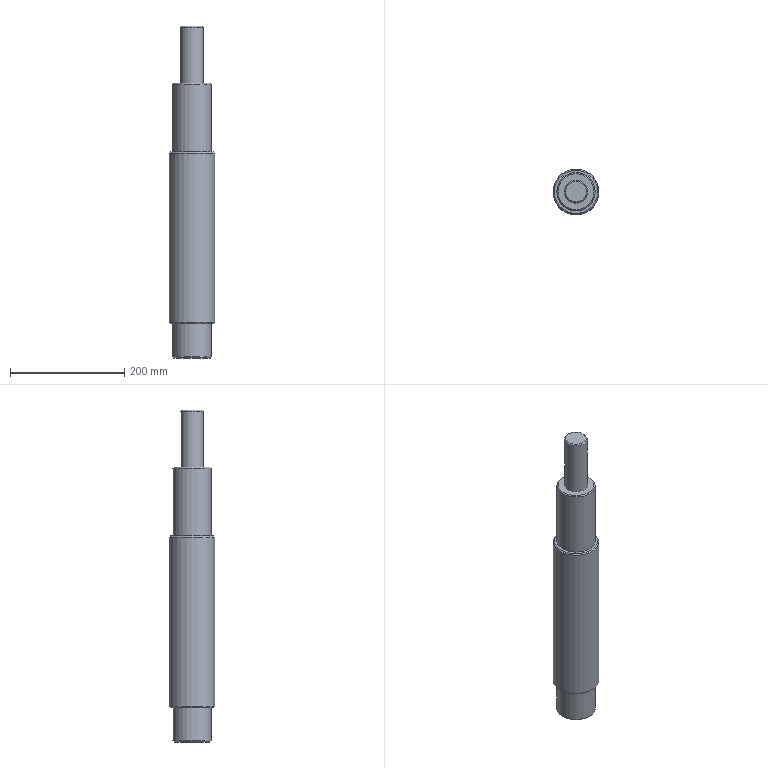Part | NX | features CYLINDER 4, CHAMFER 1, DATUM_CSYS 1 | 1 solid | 14 faces | box 80 x 80 x 580 mm | volume 2266189 mm3 | plane 5 | cone 5 | cylinder 4 | commonest cylinder face diameters 67 x2 40 x1 80 x1
STEP:
#1=CARTESIAN_POINT('',(-31.5,0.,0.));
#2=VERTEX_POINT('',#1);
#3=CARTESIAN_POINT('',(0.,0.,0.));
#4=DIRECTION('',(0.,0.,-1.));
#5=DIRECTION('',(-1.,0.,0.));
#6=AXIS2_PLACEMENT_3D('',#3,#4,#5);
#7=CIRCLE('',#6,31.5);
#8=EDGE_CURVE('',#2,#2,#7,.T.);
#9=ORIENTED_EDGE('',*,*,#8,.T.);
#10=EDGE_LOOP('',(#9));
#11=FACE_BOUND('',#10,.T.);
#12=CARTESIAN_POINT('',(0.,0.,0.));
#13=DIRECTION('',(0.,0.,-1.));
#14=DIRECTION('',(-1.,0.,0.));
#15=AXIS2_PLACEMENT_3D('',#12,#13,#14);
#16=PLANE('',#15);
#17=ADVANCED_FACE('',(#11),#16,.T.);
#18=CARTESIAN_POINT('',(-33.5,0.,2.));
#19=VERTEX_POINT('',#18);
#20=CARTESIAN_POINT('',(0.,0.,2.));
#21=DIRECTION('',(0.,0.,-1.));
#22=DIRECTION('',(-1.,0.,0.));
#23=AXIS2_PLACEMENT_3D('',#20,#21,#22);
#24=CIRCLE('',#23,33.5);
#25=EDGE_CURVE('',#19,#19,#24,.F.);
#26=ORIENTED_EDGE('',*,*,#25,.T.);
#27=EDGE_LOOP('',(#26));
#28=FACE_BOUND('',#27,.T.);
#29=CARTESIAN_POINT('',(-33.5,0.,60.));
#30=VERTEX_POINT('',#29);
#31=CARTESIAN_POINT('',(0.,0.,60.));
#32=DIRECTION('',(0.,0.,-1.));
#33=DIRECTION('',(-1.,0.,0.));
#34=AXIS2_PLACEMENT_3D('',#31,#32,#33);
#35=CIRCLE('',#34,33.5);
#36=EDGE_CURVE('',#30,#30,#35,.F.);
#37=ORIENTED_EDGE('',*,*,#36,.F.);
#38=EDGE_LOOP('',(#37));
#39=FACE_BOUND('',#38,.T.);
#40=CARTESIAN_POINT('',(0.,0.,0.));
#41=DIRECTION('',(0.,0.,1.));
#42=DIRECTION('',(1.,0.,0.));
#43=AXIS2_PLACEMENT_3D('',#40,#41,#42);
#44=CYLINDRICAL_SURFACE('',#43,33.5);
#45=ADVANCED_FACE('',(#28,#39),#44,.T.);
#46=CARTESIAN_POINT('',(38.,0.,360.));
#47=VERTEX_POINT('',#46);
#48=CARTESIAN_POINT('',(0.,0.,360.));
#49=DIRECTION('',(0.,0.,1.));
#50=DIRECTION('',(1.,0.,0.));
#51=AXIS2_PLACEMENT_3D('',#48,#49,#50);
#52=CIRCLE('',#51,38.);
#53=EDGE_CURVE('',#47,#47,#52,.T.);
#54=ORIENTED_EDGE('',*,*,#53,.T.);
#55=EDGE_LOOP('',(#54));
#56=FACE_BOUND('',#55,.T.);
#57=CARTESIAN_POINT('',(33.5,0.,360.));
#58=VERTEX_POINT('',#57);
#59=CARTESIAN_POINT('',(0.,0.,360.));
#60=DIRECTION('',(0.,0.,1.));
#61=DIRECTION('',(1.,0.,0.));
#62=AXIS2_PLACEMENT_3D('',#59,#60,#61);
#63=CIRCLE('',#62,33.5);
#64=EDGE_CURVE('',#58,#58,#63,.T.);
#65=ORIENTED_EDGE('',*,*,#64,.F.);
#66=EDGE_LOOP('',(#65));
#67=FACE_BOUND('',#66,.T.);
#68=CARTESIAN_POINT('',(0.,0.,360.));
#69=DIRECTION('',(0.,0.,1.));
#70=DIRECTION('',(1.,0.,0.));
#71=AXIS2_PLACEMENT_3D('',#68,#69,#70);
#72=PLANE('',#71);
#73=ADVANCED_FACE('',(#56,#67),#72,.T.);
#74=CARTESIAN_POINT('',(-38.,0.,60.));
#75=VERTEX_POINT('',#74);
#76=CARTESIAN_POINT('',(0.,0.,60.));
#77=DIRECTION('',(0.,0.,-1.));
#78=DIRECTION('',(-1.,0.,0.));
#79=AXIS2_PLACEMENT_3D('',#76,#77,#78);
#80=CIRCLE('',#79,38.);
#81=EDGE_CURVE('',#75,#75,#80,.T.);
#82=ORIENTED_EDGE('',*,*,#81,.T.);
#83=EDGE_LOOP('',(#82));
#84=FACE_BOUND('',#83,.T.);
#85=ORIENTED_EDGE('',*,*,#36,.T.);
#86=EDGE_LOOP('',(#85));
#87=FACE_BOUND('',#86,.T.);
#88=CARTESIAN_POINT('',(0.,0.,60.));
#89=DIRECTION('',(0.,0.,-1.));
#90=DIRECTION('',(-1.,0.,0.));
#91=AXIS2_PLACEMENT_3D('',#88,#89,#90);
#92=PLANE('',#91);
#93=ADVANCED_FACE('',(#84,#87),#92,.T.);
#94=CARTESIAN_POINT('',(40.,0.,358.));
#95=VERTEX_POINT('',#94);
#96=CARTESIAN_POINT('',(0.,0.,358.));
#97=DIRECTION('',(0.,0.,1.));
#98=DIRECTION('',(1.,0.,0.));
#99=AXIS2_PLACEMENT_3D('',#96,#97,#98);
#100=CIRCLE('',#99,40.);
#101=EDGE_CURVE('',#95,#95,#100,.F.);
#102=ORIENTED_EDGE('',*,*,#101,.T.);
#103=EDGE_LOOP('',(#102));
#104=FACE_BOUND('',#103,.T.);
#105=CARTESIAN_POINT('',(-40.,0.,62.));
#106=VERTEX_POINT('',#105);
#107=CARTESIAN_POINT('',(0.,0.,62.));
#108=DIRECTION('',(0.,0.,-1.));
#109=DIRECTION('',(-1.,0.,0.));
#110=AXIS2_PLACEMENT_3D('',#107,#108,#109);
#111=CIRCLE('',#110,40.);
#112=EDGE_CURVE('',#106,#106,#111,.F.);
#113=ORIENTED_EDGE('',*,*,#112,.T.);
#114=EDGE_LOOP('',(#113));
#115=FACE_BOUND('',#114,.T.);
#116=CARTESIAN_POINT('',(0.,0.,60.));
#117=DIRECTION('',(0.,0.,1.));
#118=DIRECTION('',(1.,0.,0.));
#119=AXIS2_PLACEMENT_3D('',#116,#117,#118);
#120=CYLINDRICAL_SURFACE('',#119,40.);
#121=ADVANCED_FACE('',(#104,#115),#120,.T.);
#122=CARTESIAN_POINT('',(31.5,0.,480.));
#123=VERTEX_POINT('',#122);
#124=CARTESIAN_POINT('',(0.,0.,480.));
#125=DIRECTION('',(0.,0.,1.));
#126=DIRECTION('',(1.,0.,0.));
#127=AXIS2_PLACEMENT_3D('',#124,#125,#126);
#128=CIRCLE('',#127,31.5);
#129=EDGE_CURVE('',#123,#123,#128,.T.);
#130=ORIENTED_EDGE('',*,*,#129,.T.);
#131=EDGE_LOOP('',(#130));
#132=FACE_BOUND('',#131,.T.);
#133=CARTESIAN_POINT('',(20.,0.,480.));
#134=VERTEX_POINT('',#133);
#135=CARTESIAN_POINT('',(0.,0.,480.));
#136=DIRECTION('',(0.,0.,1.));
#137=DIRECTION('',(1.,0.,0.));
#138=AXIS2_PLACEMENT_3D('',#135,#136,#137);
#139=CIRCLE('',#138,20.);
#140=EDGE_CURVE('',#134,#134,#139,.T.);
#141=ORIENTED_EDGE('',*,*,#140,.F.);
#142=EDGE_LOOP('',(#141));
#143=FACE_BOUND('',#142,.T.);
#144=CARTESIAN_POINT('',(0.,0.,480.));
#145=DIRECTION('',(0.,0.,1.));
#146=DIRECTION('',(1.,0.,0.));
#147=AXIS2_PLACEMENT_3D('',#144,#145,#146);
#148=PLANE('',#147);
#149=ADVANCED_FACE('',(#132,#143),#148,.T.);
#150=CARTESIAN_POINT('',(33.5,0.,478.));
#151=VERTEX_POINT('',#150);
#152=CARTESIAN_POINT('',(0.,0.,478.));
#153=DIRECTION('',(0.,0.,1.));
#154=DIRECTION('',(1.,0.,0.));
#155=AXIS2_PLACEMENT_3D('',#152,#153,#154);
#156=CIRCLE('',#155,33.5);
#157=EDGE_CURVE('',#151,#151,#156,.F.);
#158=ORIENTED_EDGE('',*,*,#157,.T.);
#159=EDGE_LOOP('',(#158));
#160=FACE_BOUND('',#159,.T.);
#161=ORIENTED_EDGE('',*,*,#64,.T.);
#162=EDGE_LOOP('',(#161));
#163=FACE_BOUND('',#162,.T.);
#164=CARTESIAN_POINT('',(0.,0.,360.));
#165=DIRECTION('',(0.,0.,1.));
#166=DIRECTION('',(1.,0.,0.));
#167=AXIS2_PLACEMENT_3D('',#164,#165,#166);
#168=CYLINDRICAL_SURFACE('',#167,33.5);
#169=ADVANCED_FACE('',(#160,#163),#168,.T.);
#170=CARTESIAN_POINT('',(18.,0.,580.));
#171=VERTEX_POINT('',#170);
#172=CARTESIAN_POINT('',(0.,0.,580.));
#173=DIRECTION('',(0.,0.,1.));
#174=DIRECTION('',(1.,0.,0.));
#175=AXIS2_PLACEMENT_3D('',#172,#173,#174);
#176=CIRCLE('',#175,18.);
#177=EDGE_CURVE('',#171,#171,#176,.T.);
#178=ORIENTED_EDGE('',*,*,#177,.T.);
#179=EDGE_LOOP('',(#178));
#180=FACE_BOUND('',#179,.T.);
#181=CARTESIAN_POINT('',(0.,0.,580.));
#182=DIRECTION('',(0.,0.,1.));
#183=DIRECTION('',(1.,0.,0.));
#184=AXIS2_PLACEMENT_3D('',#181,#182,#183);
#185=PLANE('',#184);
#186=ADVANCED_FACE('',(#180),#185,.T.);
#187=CARTESIAN_POINT('',(20.,0.,578.));
#188=VERTEX_POINT('',#187);
#189=CARTESIAN_POINT('',(0.,0.,578.));
#190=DIRECTION('',(0.,0.,1.));
#191=DIRECTION('',(1.,0.,0.));
#192=AXIS2_PLACEMENT_3D('',#189,#190,#191);
#193=CIRCLE('',#192,20.);
#194=EDGE_CURVE('',#188,#188,#193,.F.);
#195=ORIENTED_EDGE('',*,*,#194,.T.);
#196=EDGE_LOOP('',(#195));
#197=FACE_BOUND('',#196,.T.);
#198=ORIENTED_EDGE('',*,*,#140,.T.);
#199=EDGE_LOOP('',(#198));
#200=FACE_BOUND('',#199,.T.);
#201=CARTESIAN_POINT('',(0.,0.,480.));
#202=DIRECTION('',(0.,0.,1.));
#203=DIRECTION('',(1.,0.,0.));
#204=AXIS2_PLACEMENT_3D('',#201,#202,#203);
#205=CYLINDRICAL_SURFACE('',#204,20.);
#206=ADVANCED_FACE('',(#197,#200),#205,.T.);
#207=ORIENTED_EDGE('',*,*,#177,.F.);
#208=EDGE_LOOP('',(#207));
#209=FACE_BOUND('',#208,.T.);
#210=ORIENTED_EDGE('',*,*,#194,.F.);
#211=EDGE_LOOP('',(#210));
#212=FACE_BOUND('',#211,.T.);
#213=CARTESIAN_POINT('',(0.,0.,578.));
#214=DIRECTION('',(0.,0.,-1.));
#215=DIRECTION('',(-1.,0.,0.));
#216=AXIS2_PLACEMENT_3D('',#213,#214,#215);
#217=CONICAL_SURFACE('',#216,20.,0.7854);
#218=ADVANCED_FACE('',(#209,#212),#217,.T.);
#219=ORIENTED_EDGE('',*,*,#129,.F.);
#220=EDGE_LOOP('',(#219));
#221=FACE_BOUND('',#220,.T.);
#222=ORIENTED_EDGE('',*,*,#157,.F.);
#223=EDGE_LOOP('',(#222));
#224=FACE_BOUND('',#223,.T.);
#225=CARTESIAN_POINT('',(0.,0.,478.));
#226=DIRECTION('',(0.,0.,-1.));
#227=DIRECTION('',(-1.,0.,0.));
#228=AXIS2_PLACEMENT_3D('',#225,#226,#227);
#229=CONICAL_SURFACE('',#228,33.5,0.7854);
#230=ADVANCED_FACE('',(#221,#224),#229,.T.);
#231=ORIENTED_EDGE('',*,*,#53,.F.);
#232=EDGE_LOOP('',(#231));
#233=FACE_BOUND('',#232,.T.);
#234=ORIENTED_EDGE('',*,*,#101,.F.);
#235=EDGE_LOOP('',(#234));
#236=FACE_BOUND('',#235,.T.);
#237=CARTESIAN_POINT('',(0.,0.,358.));
#238=DIRECTION('',(0.,0.,-1.));
#239=DIRECTION('',(-1.,0.,0.));
#240=AXIS2_PLACEMENT_3D('',#237,#238,#239);
#241=CONICAL_SURFACE('',#240,40.,0.7854);
#242=ADVANCED_FACE('',(#233,#236),#241,.T.);
#243=ORIENTED_EDGE('',*,*,#81,.F.);
#244=EDGE_LOOP('',(#243));
#245=FACE_BOUND('',#244,.T.);
#246=ORIENTED_EDGE('',*,*,#112,.F.);
#247=EDGE_LOOP('',(#246));
#248=FACE_BOUND('',#247,.T.);
#249=CARTESIAN_POINT('',(0.,0.,62.));
#250=DIRECTION('',(0.,0.,1.));
#251=DIRECTION('',(1.,0.,0.));
#252=AXIS2_PLACEMENT_3D('',#249,#250,#251);
#253=CONICAL_SURFACE('',#252,40.,0.7854);
#254=ADVANCED_FACE('',(#245,#248),#253,.T.);
#255=ORIENTED_EDGE('',*,*,#8,.F.);
#256=EDGE_LOOP('',(#255));
#257=FACE_BOUND('',#256,.T.);
#258=ORIENTED_EDGE('',*,*,#25,.F.);
#259=EDGE_LOOP('',(#258));
#260=FACE_BOUND('',#259,.T.);
#261=CARTESIAN_POINT('',(0.,0.,2.));
#262=DIRECTION('',(0.,0.,1.));
#263=DIRECTION('',(1.,0.,0.));
#264=AXIS2_PLACEMENT_3D('',#261,#262,#263);
#265=CONICAL_SURFACE('',#264,33.5,0.7854);
#266=ADVANCED_FACE('',(#257,#260),#265,.T.);
#267=CLOSED_SHELL('',(#17,#45,#73,#93,#121,#149,#169,#186,#206,#218,#230,#242,#254,#266));
#268=MANIFOLD_SOLID_BREP('',#267);
#269=(LENGTH_UNIT()NAMED_UNIT(*)SI_UNIT(.MILLI.,.METRE.));
#270=UNCERTAINTY_MEASURE_WITH_UNIT(LENGTH_MEASURE(0.00001),#269,'','');
#271=(NAMED_UNIT(*)PLANE_ANGLE_UNIT()SI_UNIT($,.RADIAN.));
#272=(NAMED_UNIT(*)SI_UNIT($,.STERADIAN.)SOLID_ANGLE_UNIT());
#273=(GEOMETRIC_REPRESENTATION_CONTEXT(3)GLOBAL_UNCERTAINTY_ASSIGNED_CONTEXT((#270))GLOBAL_UNIT_ASSIGNED_CONTEXT((#269,#271,#272))REPRESENTATION_CONTEXT('',''));
#274=ADVANCED_BREP_SHAPE_REPRESENTATION('',(#268),#273);